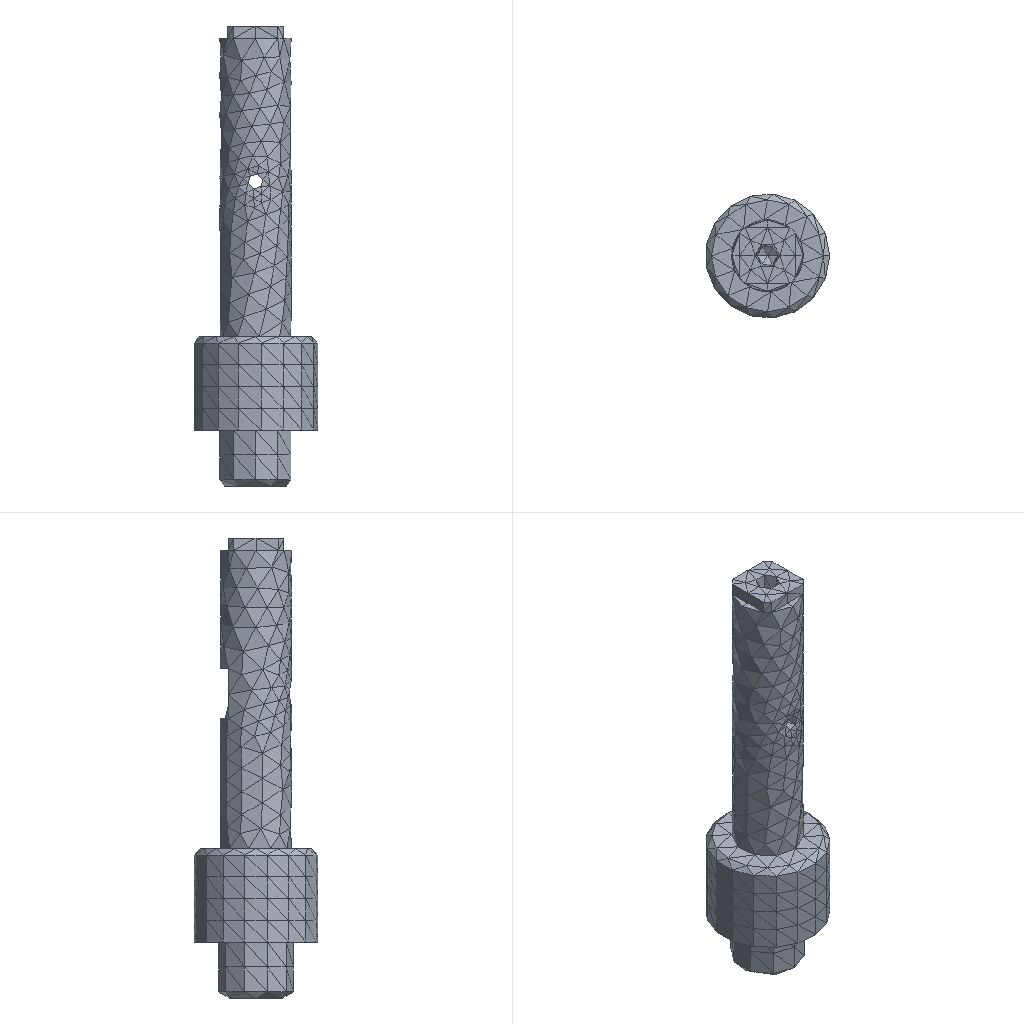Simulation study | nx simcenter
Set-up summary:
category,name,step,type,value,unit,region
solver,nx_nastran (Simcenter)
units,not stated in the deck,,not stated
analysis,deck,,static,static
analysis,solution,,SOL,101
load_step,SUBCASE 1,1,SUBCASE,SPC=1 LOAD=2
load_step,requested,,,1
mesh,nodes,,,2644
mesh,elements,,,1350
element_type,CTETRA,,solid,1350
load,nodal force total,,FX,0.0,model units
load,nodal force total,,FY,-1500000.0,model units
load,nodal force total,,FZ,0.0,model units
load,load commands in deck,,count,47
bc,support commands in deck,,count,100
analysis,NX solution 0,,Structural,Linear Statics - Single Constraint
check,setup vs results,,match,every grid point's frame and coordinates and every element id; grid points of CTETRA elements
Nastran input file, long lists of numbers shortened:
$*$$$$$$$$$$$$$$$$$$$$$$$$$$$$$$$$$$$$$$$$$$$$$$$$$$$$$$$$$$$$$$$$$
$*
$*                    NX v10.0.0.24 TRANSLATOR
$*                    FOR NX NASTRAN VERSION 10.0
$ (33 more lines like these left out)
ASSIGN OUTPUT2='151_sim1-solution_1.op2' UNIT=12
$*
$*$$$$$$$$$$$$$$$$$$$$$$$$$$$$$$$$$$$
$*
$* EXECUTIVE CONTROL
$*
$*$$$$$$$$$$$$$$$$$$$$$$$$$$$$$$$$$$$
$*
ID,NASTRAN,151_sim1-solution_1
SOL 101
CEND
$*
$*$$$$$$$$$$$$$$$$$$$$$$$$$$$$$$$$$$$
$*
$* CASE CONTROL
$*
$*$$$$$$$$$$$$$$$$$$$$$$$$$$$$$$$$$$$
$*
TITLE = Solution 1
ECHO = NONE
SPC = 1
OUTPUT
BCRESULTS(TRACTION,FORCE,PLOT) = ALL
DISPLACEMENT(PLOT) = ALL
ESE(PLOT) = ALL
FORCE(PLOT,CORNER) = ALL
OLOAD(PLOT) = ALL
SPCFORCES(PLOT) = ALL
STRAIN(PLOT,FIBER,CORNER) = ALL
STRESS(PLOT,CORNER) = ALL
$*  NX Step: Subcase - Static Loads 1
SUBCASE 1
LABEL = Subcase - Static Loads 1
LOAD = 2
$*
$*$$$$$$$$$$$$$$$$$$$$$$$$$$$$$$$$$$$
$*
$* BULK DATA
$*
$*$$$$$$$$$$$$$$$$$$$$$$$$$$$$$$$$$$$
$*
BEGIN BULK
$*
$* PARAM CARDS
$*
PARAM      K6ROT100.0000
PARAM     OIBULK     YES
PARAM    OMACHPR     YES
PARAM       POST      -2
PARAM    POSTEXT     YES
PARAM    UNITSYS   MN-MM
$*
$* GRID CARDS
$*
GRID*               2613               01.0000000000E+011.2246467996E-15+
*       9.0000000000E+00               0
GRID*               2614               01.0000000000E+011.2246467996E-15+
*       2.3000000000E+01               0
$ (5284 more lines like these left out)
$*
$* ELEMENT CARDS
$*
$*  NX Mesh Collector: Solid(1)
$*  NX Mesh: 3d_mesh(1)
CTETRA         1       1       1       2    2430    2429      60      61+
+             62      63      64    2439
CTETRA         2       1       3       4       5       1      65      66+
+             67      68      69      70
$ (2696 more lines like these left out)
$*
$* PROPERTY CARDS
$*
$*  NX Property: PSOLID1
PSOLID         1       1       0                           SMECH
$*
$* MATERIAL CARDS
$*
$*  NX Material: 7075
MAT1           12.0000+8        0.3300002.8100-62.1355-5
MATT1          1                       1               2
TABLEM1        1                                                        +
+        20.00000.330000 21.11000.330000    ENDT
TABLEM1        2                                                        +
+        20.00002.1600-5 93.33002.2500-5107.22002.2662-5121.11002.2824-5+
+       135.00002.2968-5148.89002.3130-5162.78002.3274-5176.67002.3418-5+
+       190.56002.3544-5204.44002.3688-5218.33002.3814-5232.22002.3958-5+
+       246.11002.4066-5260.00002.4192-5273.89002.4300-5287.78002.4408-5+
+       301.67002.4498-5315.56002.4606-5329.44002.4696-5343.33002.4786-5+
+       357.22002.4876-5371.11002.4984-5385.00002.5110-5398.89002.5254-5+
+       412.78002.5398-5426.67002.5560-5    ENDT
$*
$* LOAD AND CONSTRAINT CARDS
$*
$*  NX Load and Constraint: Fixed(1)
SPC            1    1399  123456  0.0000
SPC            1    1400  123456  0.0000
SPC            1    1401  123456  0.0000
SPC            1    1402  123456  0.0000
$ (96 more lines like these left out)
$*  NX Load and Constraint: Force(1)
FORCE          2    2268       057532.18  0.0000-1.00000  0.0000
FORCE          2    2269       078342.17  0.0000-1.00000  0.0000
FORCE          2    2270       027986.86  0.0000-1.00000  0.0000
FORCE          2    2271       035768.90  0.0000-1.00000  0.0000
$ (43 more lines like these left out)
ENDDATA 18ea3e19
Results summary:
result,analysis,,,static
result,last_loadstep,,,1
result,primary field,,,displacements
result,reaction total,,FX,0.0155,model units
result,reaction total,,FY,1500000.0,model units
result,reaction total,,FZ,-0.03931,model units
result,NX solution 0,,loadcases,1,mm